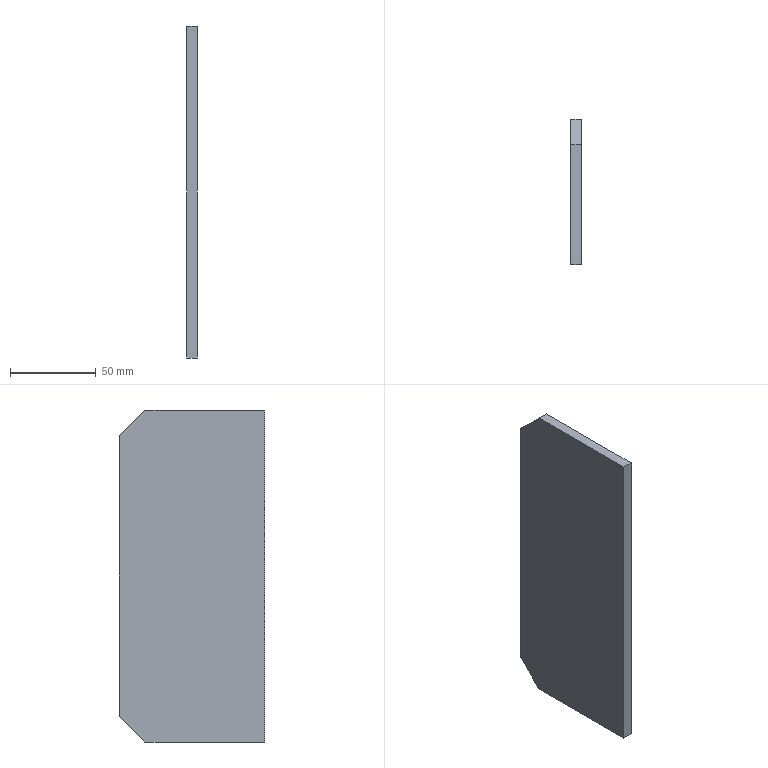Part | STEP file | 3_2_00 | 1 solid | 8 faces | box 6 x 85 x 194 mm | volume 97590 mm3 | plane 8
STEP:
#1=CARTESIAN_POINT('',(-3.,85.,-310.5));
#2=VERTEX_POINT('',#1);
#3=CARTESIAN_POINT('',(3.,85.,-310.5));
#4=VERTEX_POINT('',#3);
#5=CARTESIAN_POINT('',(-3.,85.,-310.5));
#6=DIRECTION('',(1.,0.,0.));
#7=VECTOR('',#6,1000.);
#8=LINE('',#5,#7);
#9=EDGE_CURVE('',#2,#4,#8,.T.);
#10=ORIENTED_EDGE('',*,*,#9,.T.);
#11=CARTESIAN_POINT('',(3.,70.,-325.5));
#12=VERTEX_POINT('',#11);
#13=CARTESIAN_POINT('',(3.,70.,-325.5));
#14=DIRECTION('',(0.,0.7071,0.7071));
#15=VECTOR('',#14,1000.);
#16=LINE('',#13,#15);
#17=EDGE_CURVE('',#12,#4,#16,.T.);
#18=ORIENTED_EDGE('',*,*,#17,.F.);
#19=CARTESIAN_POINT('',(-3.,70.,-325.5));
#20=VERTEX_POINT('',#19);
#21=CARTESIAN_POINT('',(-3.,70.,-325.5));
#22=DIRECTION('',(1.,0.,0.));
#23=VECTOR('',#22,1000.);
#24=LINE('',#21,#23);
#25=EDGE_CURVE('',#20,#12,#24,.T.);
#26=ORIENTED_EDGE('',*,*,#25,.F.);
#27=CARTESIAN_POINT('',(-3.,85.,-310.5));
#28=DIRECTION('',(0.,-0.7071,-0.7071));
#29=VECTOR('',#28,1000.);
#30=LINE('',#27,#29);
#31=EDGE_CURVE('',#2,#20,#30,.T.);
#32=ORIENTED_EDGE('',*,*,#31,.F.);
#33=EDGE_LOOP('',(#10,#18,#26,#32));
#34=FACE_OUTER_BOUND('',#33,.T.);
#35=CARTESIAN_POINT('',(3.,70.,-325.5));
#36=DIRECTION('',(0.,-0.7071,0.7071));
#37=DIRECTION('',(-1.,0.,0.));
#38=AXIS2_PLACEMENT_3D('',#35,#36,#37);
#39=PLANE('',#38);
#40=ADVANCED_FACE('',(#34),#39,.F.);
#41=ORIENTED_EDGE('',*,*,#17,.T.);
#42=CARTESIAN_POINT('',(3.,85.,-146.5));
#43=VERTEX_POINT('',#42);
#44=CARTESIAN_POINT('',(3.,85.,-310.5));
#45=DIRECTION('',(0.,0.,1.));
#46=VECTOR('',#45,1000.);
#47=LINE('',#44,#46);
#48=EDGE_CURVE('',#4,#43,#47,.T.);
#49=ORIENTED_EDGE('',*,*,#48,.T.);
#50=CARTESIAN_POINT('',(3.,70.,-131.5));
#51=VERTEX_POINT('',#50);
#52=CARTESIAN_POINT('',(3.,85.,-146.5));
#53=DIRECTION('',(0.,-0.7071,0.7071));
#54=VECTOR('',#53,1000.);
#55=LINE('',#52,#54);
#56=EDGE_CURVE('',#43,#51,#55,.T.);
#57=ORIENTED_EDGE('',*,*,#56,.T.);
#58=CARTESIAN_POINT('',(3.,0.,-131.5));
#59=VERTEX_POINT('',#58);
#60=CARTESIAN_POINT('',(3.,70.,-131.5));
#61=DIRECTION('',(0.,-1.,0.));
#62=VECTOR('',#61,1000.);
#63=LINE('',#60,#62);
#64=EDGE_CURVE('',#51,#59,#63,.T.);
#65=ORIENTED_EDGE('',*,*,#64,.T.);
#66=CARTESIAN_POINT('',(3.,0.,-325.5));
#67=VERTEX_POINT('',#66);
#68=CARTESIAN_POINT('',(3.,0.,-131.5));
#69=DIRECTION('',(0.,0.,-1.));
#70=VECTOR('',#69,1000.);
#71=LINE('',#68,#70);
#72=EDGE_CURVE('',#59,#67,#71,.T.);
#73=ORIENTED_EDGE('',*,*,#72,.T.);
#74=CARTESIAN_POINT('',(3.,0.,-325.5));
#75=DIRECTION('',(0.,1.,0.));
#76=VECTOR('',#75,1000.);
#77=LINE('',#74,#76);
#78=EDGE_CURVE('',#67,#12,#77,.T.);
#79=ORIENTED_EDGE('',*,*,#78,.T.);
#80=EDGE_LOOP('',(#41,#49,#57,#65,#73,#79));
#81=FACE_OUTER_BOUND('',#80,.T.);
#82=CARTESIAN_POINT('',(3.,0.,0.));
#83=DIRECTION('',(-1.,0.,0.));
#84=DIRECTION('',(0.,0.,1.));
#85=AXIS2_PLACEMENT_3D('',#82,#83,#84);
#86=PLANE('',#85);
#87=ADVANCED_FACE('',(#81),#86,.F.);
#88=CARTESIAN_POINT('',(-3.,70.,-131.5));
#89=VERTEX_POINT('',#88);
#90=CARTESIAN_POINT('',(-3.,70.,-131.5));
#91=DIRECTION('',(1.,0.,0.));
#92=VECTOR('',#91,1000.);
#93=LINE('',#90,#92);
#94=EDGE_CURVE('',#89,#51,#93,.T.);
#95=ORIENTED_EDGE('',*,*,#94,.T.);
#96=ORIENTED_EDGE('',*,*,#56,.F.);
#97=CARTESIAN_POINT('',(-3.,85.,-146.5));
#98=VERTEX_POINT('',#97);
#99=CARTESIAN_POINT('',(-3.,85.,-146.5));
#100=DIRECTION('',(1.,0.,0.));
#101=VECTOR('',#100,1000.);
#102=LINE('',#99,#101);
#103=EDGE_CURVE('',#98,#43,#102,.T.);
#104=ORIENTED_EDGE('',*,*,#103,.F.);
#105=CARTESIAN_POINT('',(-3.,70.,-131.5));
#106=DIRECTION('',(0.,0.7071,-0.7071));
#107=VECTOR('',#106,1000.);
#108=LINE('',#105,#107);
#109=EDGE_CURVE('',#89,#98,#108,.T.);
#110=ORIENTED_EDGE('',*,*,#109,.F.);
#111=EDGE_LOOP('',(#95,#96,#104,#110));
#112=FACE_OUTER_BOUND('',#111,.T.);
#113=CARTESIAN_POINT('',(3.,85.,-146.5));
#114=DIRECTION('',(0.,-0.7071,-0.7071));
#115=DIRECTION('',(0.,-0.7071,0.7071));
#116=AXIS2_PLACEMENT_3D('',#113,#114,#115);
#117=PLANE('',#116);
#118=ADVANCED_FACE('',(#112),#117,.F.);
#119=CARTESIAN_POINT('',(-3.,0.,-131.5));
#120=VERTEX_POINT('',#119);
#121=CARTESIAN_POINT('',(-3.,0.,-131.5));
#122=DIRECTION('',(1.,0.,0.));
#123=VECTOR('',#122,1000.);
#124=LINE('',#121,#123);
#125=EDGE_CURVE('',#120,#59,#124,.T.);
#126=ORIENTED_EDGE('',*,*,#125,.T.);
#127=ORIENTED_EDGE('',*,*,#64,.F.);
#128=ORIENTED_EDGE('',*,*,#94,.F.);
#129=CARTESIAN_POINT('',(-3.,70.,-131.5));
#130=DIRECTION('',(0.,-1.,0.));
#131=VECTOR('',#130,1000.);
#132=LINE('',#129,#131);
#133=EDGE_CURVE('',#89,#120,#132,.T.);
#134=ORIENTED_EDGE('',*,*,#133,.T.);
#135=EDGE_LOOP('',(#126,#127,#128,#134));
#136=FACE_OUTER_BOUND('',#135,.T.);
#137=CARTESIAN_POINT('',(3.,70.,-131.5));
#138=DIRECTION('',(0.,0.,-1.));
#139=DIRECTION('',(0.,-1.,0.));
#140=AXIS2_PLACEMENT_3D('',#137,#138,#139);
#141=PLANE('',#140);
#142=ADVANCED_FACE('',(#136),#141,.F.);
#143=CARTESIAN_POINT('',(-3.,0.,-325.5));
#144=VERTEX_POINT('',#143);
#145=CARTESIAN_POINT('',(-3.,0.,-325.5));
#146=DIRECTION('',(1.,0.,0.));
#147=VECTOR('',#146,1000.);
#148=LINE('',#145,#147);
#149=EDGE_CURVE('',#144,#67,#148,.T.);
#150=ORIENTED_EDGE('',*,*,#149,.T.);
#151=ORIENTED_EDGE('',*,*,#72,.F.);
#152=ORIENTED_EDGE('',*,*,#125,.F.);
#153=CARTESIAN_POINT('',(-3.,0.,-131.5));
#154=DIRECTION('',(0.,0.,-1.));
#155=VECTOR('',#154,1000.);
#156=LINE('',#153,#155);
#157=EDGE_CURVE('',#120,#144,#156,.T.);
#158=ORIENTED_EDGE('',*,*,#157,.T.);
#159=EDGE_LOOP('',(#150,#151,#152,#158));
#160=FACE_OUTER_BOUND('',#159,.T.);
#161=CARTESIAN_POINT('',(3.,0.,-325.5));
#162=DIRECTION('',(0.,1.,0.));
#163=DIRECTION('',(1.,0.,0.));
#164=AXIS2_PLACEMENT_3D('',#161,#162,#163);
#165=PLANE('',#164);
#166=ADVANCED_FACE('',(#160),#165,.F.);
#167=ORIENTED_EDGE('',*,*,#25,.T.);
#168=ORIENTED_EDGE('',*,*,#78,.F.);
#169=ORIENTED_EDGE('',*,*,#149,.F.);
#170=CARTESIAN_POINT('',(-3.,0.,-325.5));
#171=DIRECTION('',(0.,1.,0.));
#172=VECTOR('',#171,1000.);
#173=LINE('',#170,#172);
#174=EDGE_CURVE('',#144,#20,#173,.T.);
#175=ORIENTED_EDGE('',*,*,#174,.T.);
#176=EDGE_LOOP('',(#167,#168,#169,#175));
#177=FACE_OUTER_BOUND('',#176,.T.);
#178=CARTESIAN_POINT('',(3.,0.,-325.5));
#179=DIRECTION('',(0.,0.,1.));
#180=DIRECTION('',(1.,0.,0.));
#181=AXIS2_PLACEMENT_3D('',#178,#179,#180);
#182=PLANE('',#181);
#183=ADVANCED_FACE('',(#177),#182,.F.);
#184=ORIENTED_EDGE('',*,*,#157,.F.);
#185=ORIENTED_EDGE('',*,*,#133,.F.);
#186=ORIENTED_EDGE('',*,*,#109,.T.);
#187=CARTESIAN_POINT('',(-3.,85.,-310.5));
#188=DIRECTION('',(0.,0.,1.));
#189=VECTOR('',#188,1000.);
#190=LINE('',#187,#189);
#191=EDGE_CURVE('',#2,#98,#190,.T.);
#192=ORIENTED_EDGE('',*,*,#191,.F.);
#193=ORIENTED_EDGE('',*,*,#31,.T.);
#194=ORIENTED_EDGE('',*,*,#174,.F.);
#195=EDGE_LOOP('',(#184,#185,#186,#192,#193,#194));
#196=FACE_OUTER_BOUND('',#195,.T.);
#197=CARTESIAN_POINT('',(-3.,0.,0.));
#198=DIRECTION('',(-1.,0.,0.));
#199=DIRECTION('',(0.,0.,1.));
#200=AXIS2_PLACEMENT_3D('',#197,#198,#199);
#201=PLANE('',#200);
#202=ADVANCED_FACE('',(#196),#201,.T.);
#203=ORIENTED_EDGE('',*,*,#103,.T.);
#204=ORIENTED_EDGE('',*,*,#48,.F.);
#205=ORIENTED_EDGE('',*,*,#9,.F.);
#206=ORIENTED_EDGE('',*,*,#191,.T.);
#207=EDGE_LOOP('',(#203,#204,#205,#206));
#208=FACE_OUTER_BOUND('',#207,.T.);
#209=CARTESIAN_POINT('',(3.,85.,-310.5));
#210=DIRECTION('',(0.,-1.,0.));
#211=DIRECTION('',(0.,0.,-1.));
#212=AXIS2_PLACEMENT_3D('',#209,#210,#211);
#213=PLANE('',#212);
#214=ADVANCED_FACE('',(#208),#213,.F.);
#215=CLOSED_SHELL('',(#40,#87,#118,#142,#166,#183,#202,#214));
#216=MANIFOLD_SOLID_BREP('',#215);
#217=CARTESIAN_POINT('',(0.,0.,0.));
#218=DIRECTION('',(0.,0.,1.));
#219=DIRECTION('',(1.,0.,0.));
#220=AXIS2_PLACEMENT_3D('',#217,#218,#219);
#221=(LENGTH_UNIT()NAMED_UNIT(*)SI_UNIT(.MILLI.,.METRE.));
#222=UNCERTAINTY_MEASURE_WITH_UNIT(LENGTH_MEASURE(0.00001),#221,'','');
#223=(NAMED_UNIT(*)PLANE_ANGLE_UNIT()SI_UNIT($,.RADIAN.));
#224=(NAMED_UNIT(*)SI_UNIT($,.STERADIAN.)SOLID_ANGLE_UNIT());
#225=(GEOMETRIC_REPRESENTATION_CONTEXT(3)GLOBAL_UNCERTAINTY_ASSIGNED_CONTEXT((#222))GLOBAL_UNIT_ASSIGNED_CONTEXT((#221,#223,#224))REPRESENTATION_CONTEXT('',''));
#226=ADVANCED_BREP_SHAPE_REPRESENTATION('',(#216,#220),#225);